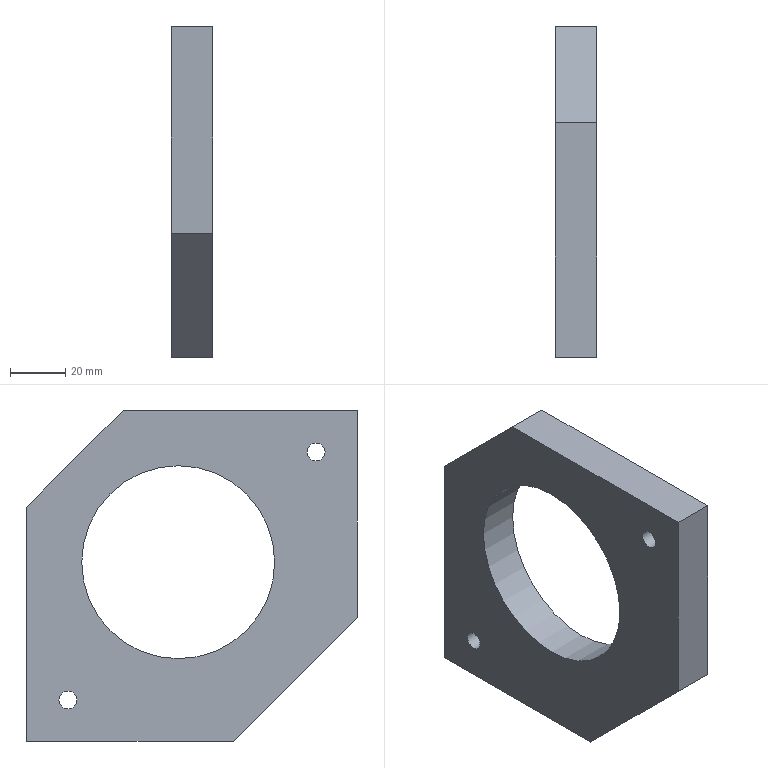Part | STEP file | solid 198 | 1 solid | 15 faces | box 15 x 120 x 120 mm | volume 132037 mm3 | plane 10 | cylinder 5 | commonest cylinder face diameters 6.5 x2 11 x2 70 x1